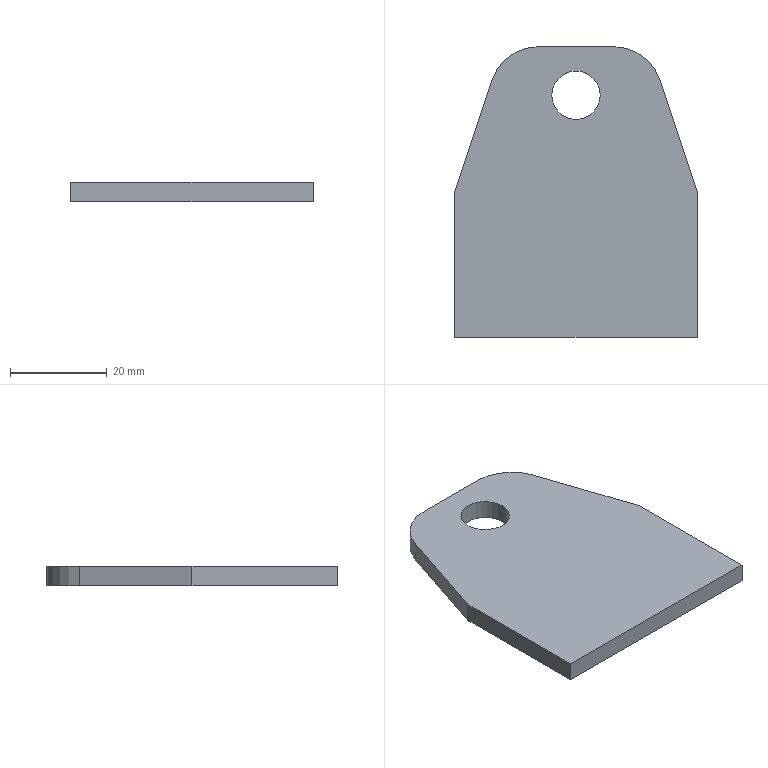Part | SolidWorks | features Extrusion 1 | 1 solid | 12 faces | box 50 x 60 x 4 mm | volume 10409 mm3 | plane 8 | cylinder 4 | commonest cylinder face diameters 10 x2 20 x2
STEP:
#1=CARTESIAN_POINT('',(20.641,18.078,4.));
#2=VERTEX_POINT('',#1);
#3=CARTESIAN_POINT('',(30.641,18.078,4.));
#4=VERTEX_POINT('',#3);
#5=CARTESIAN_POINT('',(25.641,18.078,4.));
#6=DIRECTION('',(0.,0.,1.));
#7=DIRECTION('',(1.,0.,0.));
#8=AXIS2_PLACEMENT_3D('',#5,#6,#7);
#9=CIRCLE('',#8,5.);
#10=EDGE_CURVE('',#2,#4,#9,.T.);
#11=ORIENTED_EDGE('',*,*,#10,.T.);
#12=CARTESIAN_POINT('',(30.641,18.078,0.));
#13=VERTEX_POINT('',#12);
#14=CARTESIAN_POINT('',(30.641,18.078,4.));
#15=DIRECTION('',(0.,0.,-1.));
#16=VECTOR('',#15,1000.);
#17=LINE('',#14,#16);
#18=EDGE_CURVE('',#4,#13,#17,.T.);
#19=ORIENTED_EDGE('',*,*,#18,.T.);
#20=CARTESIAN_POINT('',(20.641,18.078,0.));
#21=VERTEX_POINT('',#20);
#22=CARTESIAN_POINT('',(25.641,18.078,0.));
#23=DIRECTION('',(0.,0.,1.));
#24=DIRECTION('',(1.,0.,0.));
#25=AXIS2_PLACEMENT_3D('',#22,#23,#24);
#26=CIRCLE('',#25,5.);
#27=EDGE_CURVE('',#21,#13,#26,.T.);
#28=ORIENTED_EDGE('',*,*,#27,.F.);
#29=CARTESIAN_POINT('',(20.641,18.078,4.));
#30=DIRECTION('',(0.,0.,-1.));
#31=VECTOR('',#30,1000.);
#32=LINE('',#29,#31);
#33=EDGE_CURVE('',#2,#21,#32,.T.);
#34=ORIENTED_EDGE('',*,*,#33,.F.);
#35=EDGE_LOOP('',(#11,#19,#28,#34));
#36=FACE_OUTER_BOUND('',#35,.T.);
#37=CARTESIAN_POINT('',(25.641,18.078,4.));
#38=DIRECTION('',(0.,0.,-1.));
#39=DIRECTION('',(-1.,0.,0.));
#40=AXIS2_PLACEMENT_3D('',#37,#38,#39);
#41=CYLINDRICAL_SURFACE('',#40,5.);
#42=ADVANCED_FACE('',(#36),#41,.F.);
#43=CARTESIAN_POINT('',(0.6407,-1.922,4.));
#44=VERTEX_POINT('',#43);
#45=CARTESIAN_POINT('',(0.6407,-31.922,4.));
#46=VERTEX_POINT('',#45);
#47=CARTESIAN_POINT('',(0.6407,-1.922,4.));
#48=DIRECTION('',(0.,-1.,0.));
#49=VECTOR('',#48,1000.);
#50=LINE('',#47,#49);
#51=EDGE_CURVE('',#44,#46,#50,.T.);
#52=ORIENTED_EDGE('',*,*,#51,.T.);
#53=CARTESIAN_POINT('',(50.641,-31.922,4.));
#54=VERTEX_POINT('',#53);
#55=CARTESIAN_POINT('',(0.6407,-31.922,4.));
#56=DIRECTION('',(1.,0.,0.));
#57=VECTOR('',#56,1000.);
#58=LINE('',#55,#57);
#59=EDGE_CURVE('',#46,#54,#58,.T.);
#60=ORIENTED_EDGE('',*,*,#59,.T.);
#61=CARTESIAN_POINT('',(50.641,-1.922,4.));
#62=VERTEX_POINT('',#61);
#63=CARTESIAN_POINT('',(50.641,-1.922,4.));
#64=DIRECTION('',(0.,1.,0.));
#65=VECTOR('',#64,1000.);
#66=LINE('',#63,#65);
#67=EDGE_CURVE('',#54,#62,#66,.T.);
#68=ORIENTED_EDGE('',*,*,#67,.T.);
#69=CARTESIAN_POINT('',(42.92,21.24,4.));
#70=VERTEX_POINT('',#69);
#71=CARTESIAN_POINT('',(42.92,21.24,4.));
#72=DIRECTION('',(-0.3162,0.9487,0.));
#73=VECTOR('',#72,1000.);
#74=LINE('',#71,#73);
#75=EDGE_CURVE('',#62,#70,#74,.T.);
#76=ORIENTED_EDGE('',*,*,#75,.T.);
#77=CARTESIAN_POINT('',(33.433,28.078,4.));
#78=VERTEX_POINT('',#77);
#79=CARTESIAN_POINT('',(33.433,18.078,4.));
#80=DIRECTION('',(0.,0.,1.));
#81=DIRECTION('',(1.,0.,0.));
#82=AXIS2_PLACEMENT_3D('',#79,#80,#81);
#83=CIRCLE('',#82,10.);
#84=EDGE_CURVE('',#70,#78,#83,.T.);
#85=ORIENTED_EDGE('',*,*,#84,.T.);
#86=CARTESIAN_POINT('',(17.848,28.078,4.));
#87=VERTEX_POINT('',#86);
#88=CARTESIAN_POINT('',(33.433,28.078,4.));
#89=DIRECTION('',(-1.,0.,0.));
#90=VECTOR('',#89,1000.);
#91=LINE('',#88,#90);
#92=EDGE_CURVE('',#78,#87,#91,.T.);
#93=ORIENTED_EDGE('',*,*,#92,.T.);
#94=CARTESIAN_POINT('',(8.362,21.24,4.));
#95=VERTEX_POINT('',#94);
#96=CARTESIAN_POINT('',(17.848,18.078,4.));
#97=DIRECTION('',(0.,0.,1.));
#98=DIRECTION('',(1.,0.,0.));
#99=AXIS2_PLACEMENT_3D('',#96,#97,#98);
#100=CIRCLE('',#99,10.);
#101=EDGE_CURVE('',#87,#95,#100,.T.);
#102=ORIENTED_EDGE('',*,*,#101,.T.);
#103=CARTESIAN_POINT('',(8.362,21.24,4.));
#104=DIRECTION('',(-0.3162,-0.9487,0.));
#105=VECTOR('',#104,1000.);
#106=LINE('',#103,#105);
#107=EDGE_CURVE('',#95,#44,#106,.T.);
#108=ORIENTED_EDGE('',*,*,#107,.T.);
#109=EDGE_LOOP('',(#52,#60,#68,#76,#85,#93,#102,#108));
#110=FACE_OUTER_BOUND('',#109,.T.);
#111=ORIENTED_EDGE('',*,*,#10,.F.);
#112=CARTESIAN_POINT('',(25.641,18.078,4.));
#113=DIRECTION('',(0.,0.,1.));
#114=DIRECTION('',(1.,0.,0.));
#115=AXIS2_PLACEMENT_3D('',#112,#113,#114);
#116=CIRCLE('',#115,5.);
#117=EDGE_CURVE('',#4,#2,#116,.T.);
#118=ORIENTED_EDGE('',*,*,#117,.F.);
#119=EDGE_LOOP('',(#111,#118));
#120=FACE_BOUND('',#119,.T.);
#121=CARTESIAN_POINT('',(33.433,18.078,4.));
#122=DIRECTION('',(0.,0.,1.));
#123=DIRECTION('',(1.,0.,0.));
#124=AXIS2_PLACEMENT_3D('',#121,#122,#123);
#125=PLANE('',#124);
#126=ADVANCED_FACE('',(#110,#120),#125,.T.);
#127=CARTESIAN_POINT('',(0.6407,-1.922,0.));
#128=VERTEX_POINT('',#127);
#129=CARTESIAN_POINT('',(0.6407,-31.922,0.));
#130=VERTEX_POINT('',#129);
#131=CARTESIAN_POINT('',(0.6407,-1.922,0.));
#132=DIRECTION('',(0.,-1.,0.));
#133=VECTOR('',#132,1000.);
#134=LINE('',#131,#133);
#135=EDGE_CURVE('',#128,#130,#134,.T.);
#136=ORIENTED_EDGE('',*,*,#135,.F.);
#137=CARTESIAN_POINT('',(8.362,21.24,0.));
#138=VERTEX_POINT('',#137);
#139=CARTESIAN_POINT('',(8.362,21.24,0.));
#140=DIRECTION('',(-0.3162,-0.9487,0.));
#141=VECTOR('',#140,1000.);
#142=LINE('',#139,#141);
#143=EDGE_CURVE('',#138,#128,#142,.T.);
#144=ORIENTED_EDGE('',*,*,#143,.F.);
#145=CARTESIAN_POINT('',(17.848,28.078,0.));
#146=VERTEX_POINT('',#145);
#147=CARTESIAN_POINT('',(17.848,18.078,0.));
#148=DIRECTION('',(0.,0.,1.));
#149=DIRECTION('',(1.,0.,0.));
#150=AXIS2_PLACEMENT_3D('',#147,#148,#149);
#151=CIRCLE('',#150,10.);
#152=EDGE_CURVE('',#146,#138,#151,.T.);
#153=ORIENTED_EDGE('',*,*,#152,.F.);
#154=CARTESIAN_POINT('',(33.433,28.078,0.));
#155=VERTEX_POINT('',#154);
#156=CARTESIAN_POINT('',(33.433,28.078,0.));
#157=DIRECTION('',(-1.,0.,0.));
#158=VECTOR('',#157,1000.);
#159=LINE('',#156,#158);
#160=EDGE_CURVE('',#155,#146,#159,.T.);
#161=ORIENTED_EDGE('',*,*,#160,.F.);
#162=CARTESIAN_POINT('',(42.92,21.24,0.));
#163=VERTEX_POINT('',#162);
#164=CARTESIAN_POINT('',(33.433,18.078,0.));
#165=DIRECTION('',(0.,0.,1.));
#166=DIRECTION('',(1.,0.,0.));
#167=AXIS2_PLACEMENT_3D('',#164,#165,#166);
#168=CIRCLE('',#167,10.);
#169=EDGE_CURVE('',#163,#155,#168,.T.);
#170=ORIENTED_EDGE('',*,*,#169,.F.);
#171=CARTESIAN_POINT('',(50.641,-1.922,0.));
#172=VERTEX_POINT('',#171);
#173=CARTESIAN_POINT('',(42.92,21.24,0.));
#174=DIRECTION('',(-0.3162,0.9487,0.));
#175=VECTOR('',#174,1000.);
#176=LINE('',#173,#175);
#177=EDGE_CURVE('',#172,#163,#176,.T.);
#178=ORIENTED_EDGE('',*,*,#177,.F.);
#179=CARTESIAN_POINT('',(50.641,-31.922,0.));
#180=VERTEX_POINT('',#179);
#181=CARTESIAN_POINT('',(50.641,-1.922,0.));
#182=DIRECTION('',(0.,1.,0.));
#183=VECTOR('',#182,1000.);
#184=LINE('',#181,#183);
#185=EDGE_CURVE('',#180,#172,#184,.T.);
#186=ORIENTED_EDGE('',*,*,#185,.F.);
#187=CARTESIAN_POINT('',(0.6407,-31.922,0.));
#188=DIRECTION('',(1.,0.,0.));
#189=VECTOR('',#188,1000.);
#190=LINE('',#187,#189);
#191=EDGE_CURVE('',#130,#180,#190,.T.);
#192=ORIENTED_EDGE('',*,*,#191,.F.);
#193=EDGE_LOOP('',(#136,#144,#153,#161,#170,#178,#186,#192));
#194=FACE_OUTER_BOUND('',#193,.T.);
#195=ORIENTED_EDGE('',*,*,#27,.T.);
#196=CARTESIAN_POINT('',(25.641,18.078,0.));
#197=DIRECTION('',(0.,0.,1.));
#198=DIRECTION('',(1.,0.,0.));
#199=AXIS2_PLACEMENT_3D('',#196,#197,#198);
#200=CIRCLE('',#199,5.);
#201=EDGE_CURVE('',#13,#21,#200,.T.);
#202=ORIENTED_EDGE('',*,*,#201,.T.);
#203=EDGE_LOOP('',(#195,#202));
#204=FACE_BOUND('',#203,.T.);
#205=CARTESIAN_POINT('',(33.433,18.078,0.));
#206=DIRECTION('',(0.,0.,1.));
#207=DIRECTION('',(1.,0.,0.));
#208=AXIS2_PLACEMENT_3D('',#205,#206,#207);
#209=PLANE('',#208);
#210=ADVANCED_FACE('',(#194,#204),#209,.F.);
#211=ORIENTED_EDGE('',*,*,#135,.T.);
#212=CARTESIAN_POINT('',(0.6407,-31.922,4.));
#213=DIRECTION('',(0.,0.,-1.));
#214=VECTOR('',#213,1000.);
#215=LINE('',#212,#214);
#216=EDGE_CURVE('',#46,#130,#215,.T.);
#217=ORIENTED_EDGE('',*,*,#216,.F.);
#218=ORIENTED_EDGE('',*,*,#51,.F.);
#219=CARTESIAN_POINT('',(0.6407,-1.922,4.));
#220=DIRECTION('',(0.,0.,-1.));
#221=VECTOR('',#220,1000.);
#222=LINE('',#219,#221);
#223=EDGE_CURVE('',#44,#128,#222,.T.);
#224=ORIENTED_EDGE('',*,*,#223,.T.);
#225=EDGE_LOOP('',(#211,#217,#218,#224));
#226=FACE_OUTER_BOUND('',#225,.T.);
#227=CARTESIAN_POINT('',(0.6407,-1.922,4.));
#228=DIRECTION('',(1.,0.,0.));
#229=DIRECTION('',(0.,0.,-1.));
#230=AXIS2_PLACEMENT_3D('',#227,#228,#229);
#231=PLANE('',#230);
#232=ADVANCED_FACE('',(#226),#231,.F.);
#233=ORIENTED_EDGE('',*,*,#191,.T.);
#234=CARTESIAN_POINT('',(50.641,-31.922,4.));
#235=DIRECTION('',(0.,0.,-1.));
#236=VECTOR('',#235,1000.);
#237=LINE('',#234,#236);
#238=EDGE_CURVE('',#54,#180,#237,.T.);
#239=ORIENTED_EDGE('',*,*,#238,.F.);
#240=ORIENTED_EDGE('',*,*,#59,.F.);
#241=ORIENTED_EDGE('',*,*,#216,.T.);
#242=EDGE_LOOP('',(#233,#239,#240,#241));
#243=FACE_OUTER_BOUND('',#242,.T.);
#244=CARTESIAN_POINT('',(0.6407,-31.922,4.));
#245=DIRECTION('',(0.,1.,0.));
#246=DIRECTION('',(0.,0.,1.));
#247=AXIS2_PLACEMENT_3D('',#244,#245,#246);
#248=PLANE('',#247);
#249=ADVANCED_FACE('',(#243),#248,.F.);
#250=ORIENTED_EDGE('',*,*,#185,.T.);
#251=CARTESIAN_POINT('',(50.641,-1.922,4.));
#252=DIRECTION('',(0.,0.,-1.));
#253=VECTOR('',#252,1000.);
#254=LINE('',#251,#253);
#255=EDGE_CURVE('',#62,#172,#254,.T.);
#256=ORIENTED_EDGE('',*,*,#255,.F.);
#257=ORIENTED_EDGE('',*,*,#67,.F.);
#258=ORIENTED_EDGE('',*,*,#238,.T.);
#259=EDGE_LOOP('',(#250,#256,#257,#258));
#260=FACE_OUTER_BOUND('',#259,.T.);
#261=CARTESIAN_POINT('',(50.641,-1.922,4.));
#262=DIRECTION('',(-1.,0.,0.));
#263=DIRECTION('',(0.,0.,1.));
#264=AXIS2_PLACEMENT_3D('',#261,#262,#263);
#265=PLANE('',#264);
#266=ADVANCED_FACE('',(#260),#265,.F.);
#267=ORIENTED_EDGE('',*,*,#177,.T.);
#268=CARTESIAN_POINT('',(42.92,21.24,4.));
#269=DIRECTION('',(0.,0.,-1.));
#270=VECTOR('',#269,1000.);
#271=LINE('',#268,#270);
#272=EDGE_CURVE('',#70,#163,#271,.T.);
#273=ORIENTED_EDGE('',*,*,#272,.F.);
#274=ORIENTED_EDGE('',*,*,#75,.F.);
#275=ORIENTED_EDGE('',*,*,#255,.T.);
#276=EDGE_LOOP('',(#267,#273,#274,#275));
#277=FACE_OUTER_BOUND('',#276,.T.);
#278=CARTESIAN_POINT('',(42.92,21.24,4.));
#279=DIRECTION('',(-0.9487,-0.3162,0.));
#280=DIRECTION('',(0.3162,-0.9487,0.));
#281=AXIS2_PLACEMENT_3D('',#278,#279,#280);
#282=PLANE('',#281);
#283=ADVANCED_FACE('',(#277),#282,.F.);
#284=ORIENTED_EDGE('',*,*,#169,.T.);
#285=CARTESIAN_POINT('',(33.433,28.078,4.));
#286=DIRECTION('',(0.,0.,-1.));
#287=VECTOR('',#286,1000.);
#288=LINE('',#285,#287);
#289=EDGE_CURVE('',#78,#155,#288,.T.);
#290=ORIENTED_EDGE('',*,*,#289,.F.);
#291=ORIENTED_EDGE('',*,*,#84,.F.);
#292=ORIENTED_EDGE('',*,*,#272,.T.);
#293=EDGE_LOOP('',(#284,#290,#291,#292));
#294=FACE_OUTER_BOUND('',#293,.T.);
#295=CARTESIAN_POINT('',(33.433,18.078,4.));
#296=DIRECTION('',(0.,0.,-1.));
#297=DIRECTION('',(-1.,0.,0.));
#298=AXIS2_PLACEMENT_3D('',#295,#296,#297);
#299=CYLINDRICAL_SURFACE('',#298,10.);
#300=ADVANCED_FACE('',(#294),#299,.T.);
#301=ORIENTED_EDGE('',*,*,#160,.T.);
#302=CARTESIAN_POINT('',(17.848,28.078,4.));
#303=DIRECTION('',(0.,0.,-1.));
#304=VECTOR('',#303,1000.);
#305=LINE('',#302,#304);
#306=EDGE_CURVE('',#87,#146,#305,.T.);
#307=ORIENTED_EDGE('',*,*,#306,.F.);
#308=ORIENTED_EDGE('',*,*,#92,.F.);
#309=ORIENTED_EDGE('',*,*,#289,.T.);
#310=EDGE_LOOP('',(#301,#307,#308,#309));
#311=FACE_OUTER_BOUND('',#310,.T.);
#312=CARTESIAN_POINT('',(33.433,28.078,4.));
#313=DIRECTION('',(0.,-1.,0.));
#314=DIRECTION('',(1.,0.,0.));
#315=AXIS2_PLACEMENT_3D('',#312,#313,#314);
#316=PLANE('',#315);
#317=ADVANCED_FACE('',(#311),#316,.F.);
#318=ORIENTED_EDGE('',*,*,#152,.T.);
#319=CARTESIAN_POINT('',(8.362,21.24,4.));
#320=DIRECTION('',(0.,0.,-1.));
#321=VECTOR('',#320,1000.);
#322=LINE('',#319,#321);
#323=EDGE_CURVE('',#95,#138,#322,.T.);
#324=ORIENTED_EDGE('',*,*,#323,.F.);
#325=ORIENTED_EDGE('',*,*,#101,.F.);
#326=ORIENTED_EDGE('',*,*,#306,.T.);
#327=EDGE_LOOP('',(#318,#324,#325,#326));
#328=FACE_OUTER_BOUND('',#327,.T.);
#329=CARTESIAN_POINT('',(17.848,18.078,4.));
#330=DIRECTION('',(0.,0.,-1.));
#331=DIRECTION('',(-1.,0.,0.));
#332=AXIS2_PLACEMENT_3D('',#329,#330,#331);
#333=CYLINDRICAL_SURFACE('',#332,10.);
#334=ADVANCED_FACE('',(#328),#333,.T.);
#335=ORIENTED_EDGE('',*,*,#143,.T.);
#336=ORIENTED_EDGE('',*,*,#223,.F.);
#337=ORIENTED_EDGE('',*,*,#107,.F.);
#338=ORIENTED_EDGE('',*,*,#323,.T.);
#339=EDGE_LOOP('',(#335,#336,#337,#338));
#340=FACE_OUTER_BOUND('',#339,.T.);
#341=CARTESIAN_POINT('',(8.362,21.24,4.));
#342=DIRECTION('',(0.9487,-0.3162,0.));
#343=DIRECTION('',(0.3162,0.9487,0.));
#344=AXIS2_PLACEMENT_3D('',#341,#342,#343);
#345=PLANE('',#344);
#346=ADVANCED_FACE('',(#340),#345,.F.);
#347=ORIENTED_EDGE('',*,*,#18,.F.);
#348=ORIENTED_EDGE('',*,*,#117,.T.);
#349=ORIENTED_EDGE('',*,*,#33,.T.);
#350=ORIENTED_EDGE('',*,*,#201,.F.);
#351=EDGE_LOOP('',(#347,#348,#349,#350));
#352=FACE_OUTER_BOUND('',#351,.T.);
#353=CARTESIAN_POINT('',(25.641,18.078,4.));
#354=DIRECTION('',(0.,0.,-1.));
#355=DIRECTION('',(-1.,0.,0.));
#356=AXIS2_PLACEMENT_3D('',#353,#354,#355);
#357=CYLINDRICAL_SURFACE('',#356,5.);
#358=ADVANCED_FACE('',(#352),#357,.F.);
#359=CLOSED_SHELL('',(#42,#126,#210,#232,#249,#266,#283,#300,#317,#334,#346,#358));
#360=MANIFOLD_SOLID_BREP('',#359);
#361=CARTESIAN_POINT('',(0.,0.,0.));
#362=DIRECTION('',(0.,0.,1.));
#363=DIRECTION('',(1.,0.,0.));
#364=AXIS2_PLACEMENT_3D('',#361,#362,#363);
#365=(LENGTH_UNIT()NAMED_UNIT(*)SI_UNIT(.MILLI.,.METRE.));
#366=UNCERTAINTY_MEASURE_WITH_UNIT(LENGTH_MEASURE(0.00001),#365,'','');
#367=(NAMED_UNIT(*)PLANE_ANGLE_UNIT()SI_UNIT($,.RADIAN.));
#368=(NAMED_UNIT(*)SI_UNIT($,.STERADIAN.)SOLID_ANGLE_UNIT());
#369=(GEOMETRIC_REPRESENTATION_CONTEXT(3)GLOBAL_UNCERTAINTY_ASSIGNED_CONTEXT((#366))GLOBAL_UNIT_ASSIGNED_CONTEXT((#365,#367,#368))REPRESENTATION_CONTEXT('',''));
#370=ADVANCED_BREP_SHAPE_REPRESENTATION('',(#360,#364),#369);